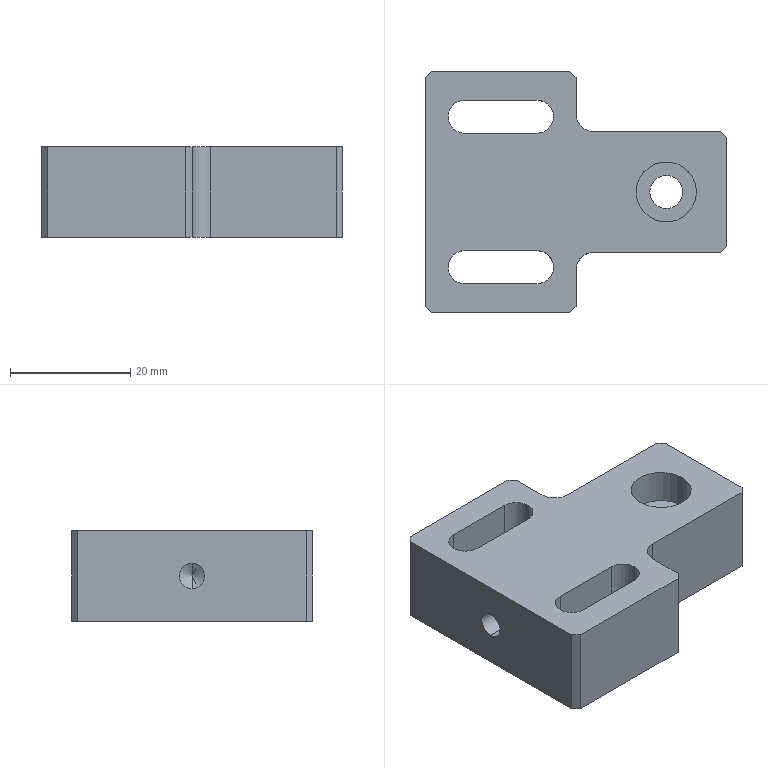Part | STEP file | MT-COMBO-119-S023 | 1 solid | 37 faces | box 50 x 40 x 15 mm | volume 18974 mm3 | plane 21 | cylinder 14 | cone 2 | commonest cylinder face diameters 5.5 x8 4.2 x2 6 x2 10 x2
STEP:
#1=CARTESIAN_POINT('',(-12.6,0.,5.4));
#2=VERTEX_POINT('',#1);
#3=CARTESIAN_POINT('',(-12.6,0.,9.6));
#4=VERTEX_POINT('',#3);
#5=CARTESIAN_POINT('',(-12.6,0.,7.5));
#6=DIRECTION('',(-1.,0.,0.));
#7=DIRECTION('',(0.,0.,1.));
#8=AXIS2_PLACEMENT_3D('',#5,#6,#7);
#9=CIRCLE('',#8,2.1);
#10=EDGE_CURVE('',#2,#4,#9,.T.);
#11=ORIENTED_EDGE('',*,*,#10,.F.);
#12=CARTESIAN_POINT('',(-25.,0.,5.4));
#13=VERTEX_POINT('',#12);
#14=CARTESIAN_POINT('',(-25.,0.,5.4));
#15=DIRECTION('',(-1.,0.,0.));
#16=VECTOR('',#15,1000.);
#17=LINE('',#14,#16);
#18=EDGE_CURVE('',#2,#13,#17,.T.);
#19=ORIENTED_EDGE('',*,*,#18,.T.);
#20=CARTESIAN_POINT('',(-25.,0.,9.6));
#21=VERTEX_POINT('',#20);
#22=CARTESIAN_POINT('',(-25.,0.,7.5));
#23=DIRECTION('',(-1.,0.,0.));
#24=DIRECTION('',(0.,0.,1.));
#25=AXIS2_PLACEMENT_3D('',#22,#23,#24);
#26=CIRCLE('',#25,2.1);
#27=EDGE_CURVE('',#13,#21,#26,.T.);
#28=ORIENTED_EDGE('',*,*,#27,.T.);
#29=CARTESIAN_POINT('',(-25.,0.,9.6));
#30=DIRECTION('',(-1.,0.,0.));
#31=VECTOR('',#30,1000.);
#32=LINE('',#29,#31);
#33=EDGE_CURVE('',#4,#21,#32,.T.);
#34=ORIENTED_EDGE('',*,*,#33,.F.);
#35=EDGE_LOOP('',(#11,#19,#28,#34));
#36=FACE_OUTER_BOUND('',#35,.T.);
#37=CARTESIAN_POINT('',(-25.,0.,7.5));
#38=DIRECTION('',(-1.,0.,0.));
#39=DIRECTION('',(0.,0.,1.));
#40=AXIS2_PLACEMENT_3D('',#37,#38,#39);
#41=CYLINDRICAL_SURFACE('',#40,2.1);
#42=ADVANCED_FACE('',(#36),#41,.F.);
#43=CARTESIAN_POINT('',(-11.338,0.,7.5));
#44=VERTEX_POINT('',#43);
#45=CARTESIAN_POINT('',(-12.6,0.,9.6));
#46=DIRECTION('',(-0.515,0.,0.8572));
#47=VECTOR('',#46,1000.);
#48=LINE('',#45,#47);
#49=EDGE_CURVE('',#44,#4,#48,.T.);
#50=ORIENTED_EDGE('',*,*,#49,.F.);
#51=CARTESIAN_POINT('',(-12.6,0.,5.4));
#52=DIRECTION('',(-0.515,0.,-0.8572));
#53=VECTOR('',#52,1000.);
#54=LINE('',#51,#53);
#55=EDGE_CURVE('',#44,#2,#54,.T.);
#56=ORIENTED_EDGE('',*,*,#55,.T.);
#57=ORIENTED_EDGE('',*,*,#10,.T.);
#58=EDGE_LOOP('',(#50,#56,#57));
#59=FACE_OUTER_BOUND('',#58,.T.);
#60=CARTESIAN_POINT('',(-12.6,0.,7.5));
#61=DIRECTION('',(-1.,0.,0.));
#62=DIRECTION('',(0.,0.,1.));
#63=AXIS2_PLACEMENT_3D('',#60,#61,#62);
#64=CONICAL_SURFACE('',#63,2.1,1.03);
#65=ADVANCED_FACE('',(#59),#64,.F.);
#66=CARTESIAN_POINT('',(-3.75,12.5,0.));
#67=VERTEX_POINT('',#66);
#68=CARTESIAN_POINT('',(-6.5,15.25,0.));
#69=VERTEX_POINT('',#68);
#70=CARTESIAN_POINT('',(-6.5,12.5,0.));
#71=DIRECTION('',(0.,0.,1.));
#72=DIRECTION('',(1.,0.,0.));
#73=AXIS2_PLACEMENT_3D('',#70,#71,#72);
#74=CIRCLE('',#73,2.75);
#75=EDGE_CURVE('',#67,#69,#74,.T.);
#76=ORIENTED_EDGE('',*,*,#75,.F.);
#77=CARTESIAN_POINT('',(-3.75,12.5,15.));
#78=VERTEX_POINT('',#77);
#79=CARTESIAN_POINT('',(-3.75,12.5,15.));
#80=DIRECTION('',(0.,0.,1.));
#81=VECTOR('',#80,1000.);
#82=LINE('',#79,#81);
#83=EDGE_CURVE('',#67,#78,#82,.T.);
#84=ORIENTED_EDGE('',*,*,#83,.T.);
#85=CARTESIAN_POINT('',(-6.5,15.25,15.));
#86=VERTEX_POINT('',#85);
#87=CARTESIAN_POINT('',(-6.5,12.5,15.));
#88=DIRECTION('',(0.,0.,1.));
#89=DIRECTION('',(1.,0.,0.));
#90=AXIS2_PLACEMENT_3D('',#87,#88,#89);
#91=CIRCLE('',#90,2.75);
#92=EDGE_CURVE('',#78,#86,#91,.T.);
#93=ORIENTED_EDGE('',*,*,#92,.T.);
#94=CARTESIAN_POINT('',(-6.5,15.25,15.));
#95=DIRECTION('',(0.,0.,1.));
#96=VECTOR('',#95,1000.);
#97=LINE('',#94,#96);
#98=EDGE_CURVE('',#69,#86,#97,.T.);
#99=ORIENTED_EDGE('',*,*,#98,.F.);
#100=EDGE_LOOP('',(#76,#84,#93,#99));
#101=FACE_OUTER_BOUND('',#100,.T.);
#102=CARTESIAN_POINT('',(-6.5,12.5,15.));
#103=DIRECTION('',(0.,0.,1.));
#104=DIRECTION('',(1.,0.,0.));
#105=AXIS2_PLACEMENT_3D('',#102,#103,#104);
#106=CYLINDRICAL_SURFACE('',#105,2.75);
#107=ADVANCED_FACE('',(#101),#106,.F.);
#108=CARTESIAN_POINT('',(-3.75,-12.5,0.));
#109=VERTEX_POINT('',#108);
#110=CARTESIAN_POINT('',(-6.5,-9.75,0.));
#111=VERTEX_POINT('',#110);
#112=CARTESIAN_POINT('',(-6.5,-12.5,0.));
#113=DIRECTION('',(0.,0.,1.));
#114=DIRECTION('',(1.,0.,0.));
#115=AXIS2_PLACEMENT_3D('',#112,#113,#114);
#116=CIRCLE('',#115,2.75);
#117=EDGE_CURVE('',#109,#111,#116,.T.);
#118=ORIENTED_EDGE('',*,*,#117,.F.);
#119=CARTESIAN_POINT('',(-3.75,-12.5,15.));
#120=VERTEX_POINT('',#119);
#121=CARTESIAN_POINT('',(-3.75,-12.5,15.));
#122=DIRECTION('',(0.,0.,1.));
#123=VECTOR('',#122,1000.);
#124=LINE('',#121,#123);
#125=EDGE_CURVE('',#109,#120,#124,.T.);
#126=ORIENTED_EDGE('',*,*,#125,.T.);
#127=CARTESIAN_POINT('',(-6.5,-9.75,15.));
#128=VERTEX_POINT('',#127);
#129=CARTESIAN_POINT('',(-6.5,-12.5,15.));
#130=DIRECTION('',(0.,0.,1.));
#131=DIRECTION('',(1.,0.,0.));
#132=AXIS2_PLACEMENT_3D('',#129,#130,#131);
#133=CIRCLE('',#132,2.75);
#134=EDGE_CURVE('',#120,#128,#133,.T.);
#135=ORIENTED_EDGE('',*,*,#134,.T.);
#136=CARTESIAN_POINT('',(-6.5,-9.75,15.));
#137=DIRECTION('',(0.,0.,1.));
#138=VECTOR('',#137,1000.);
#139=LINE('',#136,#138);
#140=EDGE_CURVE('',#111,#128,#139,.T.);
#141=ORIENTED_EDGE('',*,*,#140,.F.);
#142=EDGE_LOOP('',(#118,#126,#135,#141));
#143=FACE_OUTER_BOUND('',#142,.T.);
#144=CARTESIAN_POINT('',(-6.5,-12.5,15.));
#145=DIRECTION('',(0.,0.,1.));
#146=DIRECTION('',(1.,0.,0.));
#147=AXIS2_PLACEMENT_3D('',#144,#145,#146);
#148=CYLINDRICAL_SURFACE('',#147,2.75);
#149=ADVANCED_FACE('',(#143),#148,.F.);
#150=CARTESIAN_POINT('',(10.,0.,9.3));
#151=VERTEX_POINT('',#150);
#152=CARTESIAN_POINT('',(20.,0.,9.3));
#153=VERTEX_POINT('',#152);
#154=CARTESIAN_POINT('',(15.,0.,9.3));
#155=DIRECTION('',(0.,0.,1.));
#156=DIRECTION('',(1.,0.,0.));
#157=AXIS2_PLACEMENT_3D('',#154,#155,#156);
#158=CIRCLE('',#157,5.);
#159=EDGE_CURVE('',#151,#153,#158,.T.);
#160=ORIENTED_EDGE('',*,*,#159,.F.);
#161=CARTESIAN_POINT('',(10.,0.,15.));
#162=VERTEX_POINT('',#161);
#163=CARTESIAN_POINT('',(10.,0.,15.));
#164=DIRECTION('',(0.,0.,1.));
#165=VECTOR('',#164,1000.);
#166=LINE('',#163,#165);
#167=EDGE_CURVE('',#151,#162,#166,.T.);
#168=ORIENTED_EDGE('',*,*,#167,.T.);
#169=CARTESIAN_POINT('',(20.,0.,15.));
#170=VERTEX_POINT('',#169);
#171=CARTESIAN_POINT('',(15.,0.,15.));
#172=DIRECTION('',(0.,0.,1.));
#173=DIRECTION('',(1.,0.,0.));
#174=AXIS2_PLACEMENT_3D('',#171,#172,#173);
#175=CIRCLE('',#174,5.);
#176=EDGE_CURVE('',#162,#170,#175,.T.);
#177=ORIENTED_EDGE('',*,*,#176,.T.);
#178=CARTESIAN_POINT('',(20.,0.,15.));
#179=DIRECTION('',(0.,0.,1.));
#180=VECTOR('',#179,1000.);
#181=LINE('',#178,#180);
#182=EDGE_CURVE('',#153,#170,#181,.T.);
#183=ORIENTED_EDGE('',*,*,#182,.F.);
#184=EDGE_LOOP('',(#160,#168,#177,#183));
#185=FACE_OUTER_BOUND('',#184,.T.);
#186=CARTESIAN_POINT('',(15.,0.,15.));
#187=DIRECTION('',(0.,0.,1.));
#188=DIRECTION('',(1.,0.,0.));
#189=AXIS2_PLACEMENT_3D('',#186,#187,#188);
#190=CYLINDRICAL_SURFACE('',#189,5.);
#191=ADVANCED_FACE('',(#185),#190,.F.);
#192=CARTESIAN_POINT('',(12.25,0.,0.));
#193=VERTEX_POINT('',#192);
#194=CARTESIAN_POINT('',(17.75,0.,0.));
#195=VERTEX_POINT('',#194);
#196=CARTESIAN_POINT('',(15.,0.,0.));
#197=DIRECTION('',(0.,0.,1.));
#198=DIRECTION('',(1.,0.,0.));
#199=AXIS2_PLACEMENT_3D('',#196,#197,#198);
#200=CIRCLE('',#199,2.75);
#201=EDGE_CURVE('',#193,#195,#200,.T.);
#202=ORIENTED_EDGE('',*,*,#201,.F.);
#203=CARTESIAN_POINT('',(12.25,0.,9.3));
#204=VERTEX_POINT('',#203);
#205=CARTESIAN_POINT('',(12.25,0.,15.));
#206=DIRECTION('',(0.,0.,1.));
#207=VECTOR('',#206,1000.);
#208=LINE('',#205,#207);
#209=EDGE_CURVE('',#193,#204,#208,.T.);
#210=ORIENTED_EDGE('',*,*,#209,.T.);
#211=CARTESIAN_POINT('',(17.75,0.,9.3));
#212=VERTEX_POINT('',#211);
#213=CARTESIAN_POINT('',(15.,0.,9.3));
#214=DIRECTION('',(0.,0.,1.));
#215=DIRECTION('',(1.,0.,0.));
#216=AXIS2_PLACEMENT_3D('',#213,#214,#215);
#217=CIRCLE('',#216,2.75);
#218=EDGE_CURVE('',#204,#212,#217,.T.);
#219=ORIENTED_EDGE('',*,*,#218,.T.);
#220=CARTESIAN_POINT('',(17.75,0.,15.));
#221=DIRECTION('',(0.,0.,1.));
#222=VECTOR('',#221,1000.);
#223=LINE('',#220,#222);
#224=EDGE_CURVE('',#195,#212,#223,.T.);
#225=ORIENTED_EDGE('',*,*,#224,.F.);
#226=EDGE_LOOP('',(#202,#210,#219,#225));
#227=FACE_OUTER_BOUND('',#226,.T.);
#228=CARTESIAN_POINT('',(15.,0.,15.));
#229=DIRECTION('',(0.,0.,1.));
#230=DIRECTION('',(1.,0.,0.));
#231=AXIS2_PLACEMENT_3D('',#228,#229,#230);
#232=CYLINDRICAL_SURFACE('',#231,2.75);
#233=ADVANCED_FACE('',(#227),#232,.F.);
#234=CARTESIAN_POINT('',(25.,-9.,0.));
#235=VERTEX_POINT('',#234);
#236=CARTESIAN_POINT('',(25.,9.,0.));
#237=VERTEX_POINT('',#236);
#238=CARTESIAN_POINT('',(25.,-20.,0.));
#239=DIRECTION('',(0.,1.,0.));
#240=VECTOR('',#239,1000.);
#241=LINE('',#238,#240);
#242=EDGE_CURVE('',#235,#237,#241,.T.);
#243=ORIENTED_EDGE('',*,*,#242,.T.);
#244=CARTESIAN_POINT('',(25.,9.,15.));
#245=VERTEX_POINT('',#244);
#246=CARTESIAN_POINT('',(25.,9.,15.));
#247=DIRECTION('',(0.,0.,1.));
#248=VECTOR('',#247,1000.);
#249=LINE('',#246,#248);
#250=EDGE_CURVE('',#237,#245,#249,.T.);
#251=ORIENTED_EDGE('',*,*,#250,.T.);
#252=CARTESIAN_POINT('',(25.,-9.,15.));
#253=VERTEX_POINT('',#252);
#254=CARTESIAN_POINT('',(25.,-20.,15.));
#255=DIRECTION('',(0.,1.,0.));
#256=VECTOR('',#255,1000.);
#257=LINE('',#254,#256);
#258=EDGE_CURVE('',#253,#245,#257,.T.);
#259=ORIENTED_EDGE('',*,*,#258,.F.);
#260=CARTESIAN_POINT('',(25.,-9.,15.));
#261=DIRECTION('',(0.,0.,-1.));
#262=VECTOR('',#261,1000.);
#263=LINE('',#260,#262);
#264=EDGE_CURVE('',#253,#235,#263,.T.);
#265=ORIENTED_EDGE('',*,*,#264,.T.);
#266=EDGE_LOOP('',(#243,#251,#259,#265));
#267=FACE_OUTER_BOUND('',#266,.T.);
#268=CARTESIAN_POINT('',(25.,-20.,15.));
#269=DIRECTION('',(-1.,0.,0.));
#270=DIRECTION('',(0.,0.,1.));
#271=AXIS2_PLACEMENT_3D('',#268,#269,#270);
#272=PLANE('',#271);
#273=ADVANCED_FACE('',(#267),#272,.F.);
#274=CARTESIAN_POINT('',(-1.,20.,15.));
#275=VERTEX_POINT('',#274);
#276=CARTESIAN_POINT('',(-24.,20.,15.));
#277=VERTEX_POINT('',#276);
#278=CARTESIAN_POINT('',(-25.,20.,15.));
#279=DIRECTION('',(-1.,0.,0.));
#280=VECTOR('',#279,1000.);
#281=LINE('',#278,#280);
#282=EDGE_CURVE('',#275,#277,#281,.T.);
#283=ORIENTED_EDGE('',*,*,#282,.F.);
#284=CARTESIAN_POINT('',(-1.,20.,0.));
#285=VERTEX_POINT('',#284);
#286=CARTESIAN_POINT('',(-1.,20.,15.));
#287=DIRECTION('',(0.,0.,-1.));
#288=VECTOR('',#287,1000.);
#289=LINE('',#286,#288);
#290=EDGE_CURVE('',#275,#285,#289,.T.);
#291=ORIENTED_EDGE('',*,*,#290,.T.);
#292=CARTESIAN_POINT('',(-24.,20.,0.));
#293=VERTEX_POINT('',#292);
#294=CARTESIAN_POINT('',(-25.,20.,0.));
#295=DIRECTION('',(-1.,0.,0.));
#296=VECTOR('',#295,1000.);
#297=LINE('',#294,#296);
#298=EDGE_CURVE('',#285,#293,#297,.T.);
#299=ORIENTED_EDGE('',*,*,#298,.T.);
#300=CARTESIAN_POINT('',(-24.,20.,15.));
#301=DIRECTION('',(0.,0.,1.));
#302=VECTOR('',#301,1000.);
#303=LINE('',#300,#302);
#304=EDGE_CURVE('',#293,#277,#303,.T.);
#305=ORIENTED_EDGE('',*,*,#304,.T.);
#306=EDGE_LOOP('',(#283,#291,#299,#305));
#307=FACE_OUTER_BOUND('',#306,.T.);
#308=CARTESIAN_POINT('',(-25.,20.,15.));
#309=DIRECTION('',(0.,-1.,0.));
#310=DIRECTION('',(0.,0.,-1.));
#311=AXIS2_PLACEMENT_3D('',#308,#309,#310);
#312=PLANE('',#311);
#313=ADVANCED_FACE('',(#307),#312,.F.);
#314=CARTESIAN_POINT('',(-25.,0.,7.5));
#315=DIRECTION('',(-1.,0.,0.));
#316=DIRECTION('',(0.,0.,1.));
#317=AXIS2_PLACEMENT_3D('',#314,#315,#316);
#318=CIRCLE('',#317,2.1);
#319=EDGE_CURVE('',#21,#13,#318,.T.);
#320=ORIENTED_EDGE('',*,*,#319,.F.);
#321=ORIENTED_EDGE('',*,*,#27,.F.);
#322=EDGE_LOOP('',(#320,#321));
#323=FACE_BOUND('',#322,.T.);
#324=CARTESIAN_POINT('',(-25.,19.,15.));
#325=VERTEX_POINT('',#324);
#326=CARTESIAN_POINT('',(-25.,-19.,15.));
#327=VERTEX_POINT('',#326);
#328=CARTESIAN_POINT('',(-25.,-20.,15.));
#329=DIRECTION('',(0.,-1.,0.));
#330=VECTOR('',#329,1000.);
#331=LINE('',#328,#330);
#332=EDGE_CURVE('',#325,#327,#331,.T.);
#333=ORIENTED_EDGE('',*,*,#332,.F.);
#334=CARTESIAN_POINT('',(-25.,19.,0.));
#335=VERTEX_POINT('',#334);
#336=CARTESIAN_POINT('',(-25.,19.,15.));
#337=DIRECTION('',(0.,0.,-1.));
#338=VECTOR('',#337,1000.);
#339=LINE('',#336,#338);
#340=EDGE_CURVE('',#325,#335,#339,.T.);
#341=ORIENTED_EDGE('',*,*,#340,.T.);
#342=CARTESIAN_POINT('',(-25.,-19.,0.));
#343=VERTEX_POINT('',#342);
#344=CARTESIAN_POINT('',(-25.,-20.,0.));
#345=DIRECTION('',(0.,-1.,0.));
#346=VECTOR('',#345,1000.);
#347=LINE('',#344,#346);
#348=EDGE_CURVE('',#335,#343,#347,.T.);
#349=ORIENTED_EDGE('',*,*,#348,.T.);
#350=CARTESIAN_POINT('',(-25.,-19.,15.));
#351=DIRECTION('',(0.,0.,1.));
#352=VECTOR('',#351,1000.);
#353=LINE('',#350,#352);
#354=EDGE_CURVE('',#343,#327,#353,.T.);
#355=ORIENTED_EDGE('',*,*,#354,.T.);
#356=EDGE_LOOP('',(#333,#341,#349,#355));
#357=FACE_OUTER_BOUND('',#356,.T.);
#358=CARTESIAN_POINT('',(-25.,-20.,15.));
#359=DIRECTION('',(1.,0.,0.));
#360=DIRECTION('',(0.,0.,-1.));
#361=AXIS2_PLACEMENT_3D('',#358,#359,#360);
#362=PLANE('',#361);
#363=ADVANCED_FACE('',(#323,#357),#362,.F.);
#364=CARTESIAN_POINT('',(-24.,-20.,0.));
#365=VERTEX_POINT('',#364);
#366=CARTESIAN_POINT('',(-1.,-20.,0.));
#367=VERTEX_POINT('',#366);
#368=CARTESIAN_POINT('',(-25.,-20.,0.));
#369=DIRECTION('',(1.,0.,0.));
#370=VECTOR('',#369,1000.);
#371=LINE('',#368,#370);
#372=EDGE_CURVE('',#365,#367,#371,.T.);
#373=ORIENTED_EDGE('',*,*,#372,.T.);
#374=CARTESIAN_POINT('',(-1.,-20.,15.));
#375=VERTEX_POINT('',#374);
#376=CARTESIAN_POINT('',(-1.,-20.,15.));
#377=DIRECTION('',(0.,0.,1.));
#378=VECTOR('',#377,1000.);
#379=LINE('',#376,#378);
#380=EDGE_CURVE('',#367,#375,#379,.T.);
#381=ORIENTED_EDGE('',*,*,#380,.T.);
#382=CARTESIAN_POINT('',(-24.,-20.,15.));
#383=VERTEX_POINT('',#382);
#384=CARTESIAN_POINT('',(-25.,-20.,15.));
#385=DIRECTION('',(1.,0.,0.));
#386=VECTOR('',#385,1000.);
#387=LINE('',#384,#386);
#388=EDGE_CURVE('',#383,#375,#387,.T.);
#389=ORIENTED_EDGE('',*,*,#388,.F.);
#390=CARTESIAN_POINT('',(-24.,-20.,15.));
#391=DIRECTION('',(0.,0.,-1.));
#392=VECTOR('',#391,1000.);
#393=LINE('',#390,#392);
#394=EDGE_CURVE('',#383,#365,#393,.T.);
#395=ORIENTED_EDGE('',*,*,#394,.T.);
#396=EDGE_LOOP('',(#373,#381,#389,#395));
#397=FACE_OUTER_BOUND('',#396,.T.);
#398=CARTESIAN_POINT('',(-25.,-20.,15.));
#399=DIRECTION('',(0.,1.,0.));
#400=DIRECTION('',(0.,0.,1.));
#401=AXIS2_PLACEMENT_3D('',#398,#399,#400);
#402=PLANE('',#401);
#403=ADVANCED_FACE('',(#397),#402,.F.);
#404=CARTESIAN_POINT('',(-18.5,15.25,15.));
#405=VERTEX_POINT('',#404);
#406=CARTESIAN_POINT('',(-18.5,9.75,15.));
#407=VERTEX_POINT('',#406);
#408=CARTESIAN_POINT('',(-18.5,12.5,15.));
#409=DIRECTION('',(0.,0.,1.));
#410=DIRECTION('',(1.,0.,0.));
#411=AXIS2_PLACEMENT_3D('',#408,#409,#410);
#412=CIRCLE('',#411,2.75);
#413=EDGE_CURVE('',#405,#407,#412,.T.);
#414=ORIENTED_EDGE('',*,*,#413,.F.);
#415=CARTESIAN_POINT('',(-18.5,15.25,15.));
#416=DIRECTION('',(1.,0.,0.));
#417=VECTOR('',#416,1000.);
#418=LINE('',#415,#417);
#419=EDGE_CURVE('',#405,#86,#418,.T.);
#420=ORIENTED_EDGE('',*,*,#419,.T.);
#421=ORIENTED_EDGE('',*,*,#92,.F.);
#422=CARTESIAN_POINT('',(-6.5,9.75,15.));
#423=VERTEX_POINT('',#422);
#424=CARTESIAN_POINT('',(-6.5,12.5,15.));
#425=DIRECTION('',(0.,0.,1.));
#426=DIRECTION('',(1.,0.,0.));
#427=AXIS2_PLACEMENT_3D('',#424,#425,#426);
#428=CIRCLE('',#427,2.75);
#429=EDGE_CURVE('',#423,#78,#428,.T.);
#430=ORIENTED_EDGE('',*,*,#429,.F.);
#431=CARTESIAN_POINT('',(-18.5,9.75,15.));
#432=DIRECTION('',(1.,0.,0.));
#433=VECTOR('',#432,1000.);
#434=LINE('',#431,#433);
#435=EDGE_CURVE('',#407,#423,#434,.T.);
#436=ORIENTED_EDGE('',*,*,#435,.F.);
#437=EDGE_LOOP('',(#414,#420,#421,#430,#436));
#438=FACE_BOUND('',#437,.T.);
#439=CARTESIAN_POINT('',(-18.5,-9.75,15.));
#440=VERTEX_POINT('',#439);
#441=CARTESIAN_POINT('',(-18.5,-15.25,15.));
#442=VERTEX_POINT('',#441);
#443=CARTESIAN_POINT('',(-18.5,-12.5,15.));
#444=DIRECTION('',(0.,0.,1.));
#445=DIRECTION('',(1.,0.,0.));
#446=AXIS2_PLACEMENT_3D('',#443,#444,#445);
#447=CIRCLE('',#446,2.75);
#448=EDGE_CURVE('',#440,#442,#447,.T.);
#449=ORIENTED_EDGE('',*,*,#448,.F.);
#450=CARTESIAN_POINT('',(-18.5,-9.75,15.));
#451=DIRECTION('',(1.,0.,0.));
#452=VECTOR('',#451,1000.);
#453=LINE('',#450,#452);
#454=EDGE_CURVE('',#440,#128,#453,.T.);
#455=ORIENTED_EDGE('',*,*,#454,.T.);
#456=ORIENTED_EDGE('',*,*,#134,.F.);
#457=CARTESIAN_POINT('',(-6.5,-15.25,15.));
#458=VERTEX_POINT('',#457);
#459=CARTESIAN_POINT('',(-6.5,-12.5,15.));
#460=DIRECTION('',(0.,0.,1.));
#461=DIRECTION('',(1.,0.,0.));
#462=AXIS2_PLACEMENT_3D('',#459,#460,#461);
#463=CIRCLE('',#462,2.75);
#464=EDGE_CURVE('',#458,#120,#463,.T.);
#465=ORIENTED_EDGE('',*,*,#464,.F.);
#466=CARTESIAN_POINT('',(-18.5,-15.25,15.));
#467=DIRECTION('',(1.,0.,0.));
#468=VECTOR('',#467,1000.);
#469=LINE('',#466,#468);
#470=EDGE_CURVE('',#442,#458,#469,.T.);
#471=ORIENTED_EDGE('',*,*,#470,.F.);
#472=EDGE_LOOP('',(#449,#455,#456,#465,#471));
#473=FACE_BOUND('',#472,.T.);
#474=CARTESIAN_POINT('',(15.,0.,15.));
#475=DIRECTION('',(0.,0.,1.));
#476=DIRECTION('',(1.,0.,0.));
#477=AXIS2_PLACEMENT_3D('',#474,#475,#476);
#478=CIRCLE('',#477,5.);
#479=EDGE_CURVE('',#170,#162,#478,.T.);
#480=ORIENTED_EDGE('',*,*,#479,.F.);
#481=ORIENTED_EDGE('',*,*,#176,.F.);
#482=EDGE_LOOP('',(#480,#481));
#483=FACE_BOUND('',#482,.T.);
#484=CARTESIAN_POINT('',(0.,19.,15.));
#485=VERTEX_POINT('',#484);
#486=CARTESIAN_POINT('',(0.,13.,15.));
#487=VERTEX_POINT('',#486);
#488=CARTESIAN_POINT('',(0.,20.,15.));
#489=DIRECTION('',(0.,-1.,0.));
#490=VECTOR('',#489,1000.);
#491=LINE('',#488,#490);
#492=EDGE_CURVE('',#485,#487,#491,.T.);
#493=ORIENTED_EDGE('',*,*,#492,.F.);
#494=CARTESIAN_POINT('',(0.,19.,15.));
#495=DIRECTION('',(-0.7071,0.7071,0.));
#496=VECTOR('',#495,1000.);
#497=LINE('',#494,#496);
#498=EDGE_CURVE('',#485,#275,#497,.T.);
#499=ORIENTED_EDGE('',*,*,#498,.T.);
#500=ORIENTED_EDGE('',*,*,#282,.T.);
#501=CARTESIAN_POINT('',(-25.,19.,15.));
#502=DIRECTION('',(-0.7071,-0.7071,0.));
#503=VECTOR('',#502,1000.);
#504=LINE('',#501,#503);
#505=EDGE_CURVE('',#277,#325,#504,.T.);
#506=ORIENTED_EDGE('',*,*,#505,.T.);
#507=ORIENTED_EDGE('',*,*,#332,.T.);
#508=CARTESIAN_POINT('',(-24.,-20.,15.));
#509=DIRECTION('',(0.7071,-0.7071,0.));
#510=VECTOR('',#509,1000.);
#511=LINE('',#508,#510);
#512=EDGE_CURVE('',#327,#383,#511,.T.);
#513=ORIENTED_EDGE('',*,*,#512,.T.);
#514=ORIENTED_EDGE('',*,*,#388,.T.);
#515=CARTESIAN_POINT('',(0.,-19.,15.));
#516=VERTEX_POINT('',#515);
#517=CARTESIAN_POINT('',(-1.,-20.,15.));
#518=DIRECTION('',(0.7071,0.7071,0.));
#519=VECTOR('',#518,1000.);
#520=LINE('',#517,#519);
#521=EDGE_CURVE('',#375,#516,#520,.T.);
#522=ORIENTED_EDGE('',*,*,#521,.T.);
#523=CARTESIAN_POINT('',(0.,-13.,15.));
#524=VERTEX_POINT('',#523);
#525=CARTESIAN_POINT('',(0.,-20.,15.));
#526=DIRECTION('',(0.,-1.,0.));
#527=VECTOR('',#526,1000.);
#528=LINE('',#525,#527);
#529=EDGE_CURVE('',#524,#516,#528,.T.);
#530=ORIENTED_EDGE('',*,*,#529,.F.);
#531=CARTESIAN_POINT('',(3.,-10.,15.));
#532=VERTEX_POINT('',#531);
#533=CARTESIAN_POINT('',(3.,-13.,15.));
#534=DIRECTION('',(0.,0.,-1.));
#535=DIRECTION('',(-1.,0.,0.));
#536=AXIS2_PLACEMENT_3D('',#533,#534,#535);
#537=CIRCLE('',#536,3.);
#538=EDGE_CURVE('',#524,#532,#537,.T.);
#539=ORIENTED_EDGE('',*,*,#538,.T.);
#540=CARTESIAN_POINT('',(24.,-10.,15.));
#541=VERTEX_POINT('',#540);
#542=CARTESIAN_POINT('',(25.,-10.,15.));
#543=DIRECTION('',(-1.,0.,0.));
#544=VECTOR('',#543,1000.);
#545=LINE('',#542,#544);
#546=EDGE_CURVE('',#541,#532,#545,.T.);
#547=ORIENTED_EDGE('',*,*,#546,.F.);
#548=CARTESIAN_POINT('',(24.,-10.,15.));
#549=DIRECTION('',(0.7071,0.7071,0.));
#550=VECTOR('',#549,1000.);
#551=LINE('',#548,#550);
#552=EDGE_CURVE('',#541,#253,#551,.T.);
#553=ORIENTED_EDGE('',*,*,#552,.T.);
#554=ORIENTED_EDGE('',*,*,#258,.T.);
#555=CARTESIAN_POINT('',(24.,10.,15.));
#556=VERTEX_POINT('',#555);
#557=CARTESIAN_POINT('',(25.,9.,15.));
#558=DIRECTION('',(-0.7071,0.7071,0.));
#559=VECTOR('',#558,1000.);
#560=LINE('',#557,#559);
#561=EDGE_CURVE('',#245,#556,#560,.T.);
#562=ORIENTED_EDGE('',*,*,#561,.T.);
#563=CARTESIAN_POINT('',(3.,10.,15.));
#564=VERTEX_POINT('',#563);
#565=CARTESIAN_POINT('',(25.,10.,15.));
#566=DIRECTION('',(1.,0.,0.));
#567=VECTOR('',#566,1000.);
#568=LINE('',#565,#567);
#569=EDGE_CURVE('',#564,#556,#568,.T.);
#570=ORIENTED_EDGE('',*,*,#569,.F.);
#571=CARTESIAN_POINT('',(3.,13.,15.));
#572=DIRECTION('',(0.,0.,-1.));
#573=DIRECTION('',(-1.,0.,0.));
#574=AXIS2_PLACEMENT_3D('',#571,#572,#573);
#575=CIRCLE('',#574,3.);
#576=EDGE_CURVE('',#564,#487,#575,.T.);
#577=ORIENTED_EDGE('',*,*,#576,.T.);
#578=EDGE_LOOP('',(#493,#499,#500,#506,#507,#513,#514,#522,#530,#539,#547,#553,#554,#562,#570,#577));
#579=FACE_OUTER_BOUND('',#578,.T.);
#580=CARTESIAN_POINT('',(0.,0.,15.));
#581=DIRECTION('',(0.,0.,-1.));
#582=DIRECTION('',(-1.,0.,0.));
#583=AXIS2_PLACEMENT_3D('',#580,#581,#582);
#584=PLANE('',#583);
#585=ADVANCED_FACE('',(#438,#473,#483,#579),#584,.F.);
#586=CARTESIAN_POINT('',(-18.5,15.25,0.));
#587=VERTEX_POINT('',#586);
#588=CARTESIAN_POINT('',(-18.5,15.25,0.));
#589=DIRECTION('',(1.,0.,0.));
#590=VECTOR('',#589,1000.);
#591=LINE('',#588,#590);
#592=EDGE_CURVE('',#587,#69,#591,.T.);
#593=ORIENTED_EDGE('',*,*,#592,.F.);
#594=CARTESIAN_POINT('',(-18.5,9.75,0.));
#595=VERTEX_POINT('',#594);
#596=CARTESIAN_POINT('',(-18.5,12.5,0.));
#597=DIRECTION('',(0.,0.,1.));
#598=DIRECTION('',(1.,0.,0.));
#599=AXIS2_PLACEMENT_3D('',#596,#597,#598);
#600=CIRCLE('',#599,2.75);
#601=EDGE_CURVE('',#587,#595,#600,.T.);
#602=ORIENTED_EDGE('',*,*,#601,.T.);
#603=CARTESIAN_POINT('',(-6.5,9.75,0.));
#604=VERTEX_POINT('',#603);
#605=CARTESIAN_POINT('',(-18.5,9.75,0.));
#606=DIRECTION('',(1.,0.,0.));
#607=VECTOR('',#606,1000.);
#608=LINE('',#605,#607);
#609=EDGE_CURVE('',#595,#604,#608,.T.);
#610=ORIENTED_EDGE('',*,*,#609,.T.);
#611=CARTESIAN_POINT('',(-6.5,12.5,0.));
#612=DIRECTION('',(0.,0.,1.));
#613=DIRECTION('',(1.,0.,0.));
#614=AXIS2_PLACEMENT_3D('',#611,#612,#613);
#615=CIRCLE('',#614,2.75);
#616=EDGE_CURVE('',#604,#67,#615,.T.);
#617=ORIENTED_EDGE('',*,*,#616,.T.);
#618=ORIENTED_EDGE('',*,*,#75,.T.);
#619=EDGE_LOOP('',(#593,#602,#610,#617,#618));
#620=FACE_BOUND('',#619,.T.);
#621=CARTESIAN_POINT('',(-6.5,-15.25,0.));
#622=VERTEX_POINT('',#621);
#623=CARTESIAN_POINT('',(-6.5,-12.5,0.));
#624=DIRECTION('',(0.,0.,1.));
#625=DIRECTION('',(1.,0.,0.));
#626=AXIS2_PLACEMENT_3D('',#623,#624,#625);
#627=CIRCLE('',#626,2.75);
#628=EDGE_CURVE('',#622,#109,#627,.T.);
#629=ORIENTED_EDGE('',*,*,#628,.T.);
#630=ORIENTED_EDGE('',*,*,#117,.T.);
#631=CARTESIAN_POINT('',(-18.5,-9.75,0.));
#632=VERTEX_POINT('',#631);
#633=CARTESIAN_POINT('',(-18.5,-9.75,0.));
#634=DIRECTION('',(1.,0.,0.));
#635=VECTOR('',#634,1000.);
#636=LINE('',#633,#635);
#637=EDGE_CURVE('',#632,#111,#636,.T.);
#638=ORIENTED_EDGE('',*,*,#637,.F.);
#639=CARTESIAN_POINT('',(-18.5,-15.25,0.));
#640=VERTEX_POINT('',#639);
#641=CARTESIAN_POINT('',(-18.5,-12.5,0.));
#642=DIRECTION('',(0.,0.,1.));
#643=DIRECTION('',(1.,0.,0.));
#644=AXIS2_PLACEMENT_3D('',#641,#642,#643);
#645=CIRCLE('',#644,2.75);
#646=EDGE_CURVE('',#632,#640,#645,.T.);
#647=ORIENTED_EDGE('',*,*,#646,.T.);
#648=CARTESIAN_POINT('',(-18.5,-15.25,0.));
#649=DIRECTION('',(1.,0.,0.));
#650=VECTOR('',#649,1000.);
#651=LINE('',#648,#650);
#652=EDGE_CURVE('',#640,#622,#651,.T.);
#653=ORIENTED_EDGE('',*,*,#652,.T.);
#654=EDGE_LOOP('',(#629,#630,#638,#647,#653));
#655=FACE_BOUND('',#654,.T.);
#656=ORIENTED_EDGE('',*,*,#298,.F.);
#657=CARTESIAN_POINT('',(0.,19.,0.));
#658=VERTEX_POINT('',#657);
#659=CARTESIAN_POINT('',(9.5,9.5,0.));
#660=DIRECTION('',(0.7071,-0.7071,0.));
#661=VECTOR('',#660,1000.);
#662=LINE('',#659,#661);
#663=EDGE_CURVE('',#285,#658,#662,.T.);
#664=ORIENTED_EDGE('',*,*,#663,.T.);
#665=CARTESIAN_POINT('',(0.,13.,0.));
#666=VERTEX_POINT('',#665);
#667=CARTESIAN_POINT('',(0.,20.,0.));
#668=DIRECTION('',(0.,-1.,0.));
#669=VECTOR('',#668,1000.);
#670=LINE('',#667,#669);
#671=EDGE_CURVE('',#658,#666,#670,.T.);
#672=ORIENTED_EDGE('',*,*,#671,.T.);
#673=CARTESIAN_POINT('',(3.,10.,0.));
#674=VERTEX_POINT('',#673);
#675=CARTESIAN_POINT('',(3.,13.,0.));
#676=DIRECTION('',(0.,0.,1.));
#677=DIRECTION('',(-1.,0.,0.));
#678=AXIS2_PLACEMENT_3D('',#675,#676,#677);
#679=CIRCLE('',#678,3.);
#680=EDGE_CURVE('',#666,#674,#679,.T.);
#681=ORIENTED_EDGE('',*,*,#680,.T.);
#682=CARTESIAN_POINT('',(24.,10.,0.));
#683=VERTEX_POINT('',#682);
#684=CARTESIAN_POINT('',(25.,10.,0.));
#685=DIRECTION('',(1.,0.,0.));
#686=VECTOR('',#685,1000.);
#687=LINE('',#684,#686);
#688=EDGE_CURVE('',#674,#683,#687,.T.);
#689=ORIENTED_EDGE('',*,*,#688,.T.);
#690=CARTESIAN_POINT('',(17.,17.,0.));
#691=DIRECTION('',(0.7071,-0.7071,0.));
#692=VECTOR('',#691,1000.);
#693=LINE('',#690,#692);
#694=EDGE_CURVE('',#683,#237,#693,.T.);
#695=ORIENTED_EDGE('',*,*,#694,.T.);
#696=ORIENTED_EDGE('',*,*,#242,.F.);
#697=CARTESIAN_POINT('',(24.,-10.,0.));
#698=VERTEX_POINT('',#697);
#699=CARTESIAN_POINT('',(17.,-17.,0.));
#700=DIRECTION('',(-0.7071,-0.7071,0.));
#701=VECTOR('',#700,1000.);
#702=LINE('',#699,#701);
#703=EDGE_CURVE('',#235,#698,#702,.T.);
#704=ORIENTED_EDGE('',*,*,#703,.T.);
#705=CARTESIAN_POINT('',(3.,-10.,0.));
#706=VERTEX_POINT('',#705);
#707=CARTESIAN_POINT('',(25.,-10.,0.));
#708=DIRECTION('',(-1.,0.,0.));
#709=VECTOR('',#708,1000.);
#710=LINE('',#707,#709);
#711=EDGE_CURVE('',#698,#706,#710,.T.);
#712=ORIENTED_EDGE('',*,*,#711,.T.);
#713=CARTESIAN_POINT('',(0.,-13.,0.));
#714=VERTEX_POINT('',#713);
#715=CARTESIAN_POINT('',(3.,-13.,0.));
#716=DIRECTION('',(0.,0.,1.));
#717=DIRECTION('',(-1.,0.,0.));
#718=AXIS2_PLACEMENT_3D('',#715,#716,#717);
#719=CIRCLE('',#718,3.);
#720=EDGE_CURVE('',#706,#714,#719,.T.);
#721=ORIENTED_EDGE('',*,*,#720,.T.);
#722=CARTESIAN_POINT('',(0.,-19.,0.));
#723=VERTEX_POINT('',#722);
#724=CARTESIAN_POINT('',(0.,-20.,0.));
#725=DIRECTION('',(0.,-1.,0.));
#726=VECTOR('',#725,1000.);
#727=LINE('',#724,#726);
#728=EDGE_CURVE('',#714,#723,#727,.T.);
#729=ORIENTED_EDGE('',*,*,#728,.T.);
#730=CARTESIAN_POINT('',(9.5,-9.5,0.));
#731=DIRECTION('',(-0.7071,-0.7071,0.));
#732=VECTOR('',#731,1000.);
#733=LINE('',#730,#732);
#734=EDGE_CURVE('',#723,#367,#733,.T.);
#735=ORIENTED_EDGE('',*,*,#734,.T.);
#736=ORIENTED_EDGE('',*,*,#372,.F.);
#737=CARTESIAN_POINT('',(-22.,-22.,0.));
#738=DIRECTION('',(-0.7071,0.7071,0.));
#739=VECTOR('',#738,1000.);
#740=LINE('',#737,#739);
#741=EDGE_CURVE('',#365,#343,#740,.T.);
#742=ORIENTED_EDGE('',*,*,#741,.T.);
#743=ORIENTED_EDGE('',*,*,#348,.F.);
#744=CARTESIAN_POINT('',(-22.,22.,0.));
#745=DIRECTION('',(0.7071,0.7071,0.));
#746=VECTOR('',#745,1000.);
#747=LINE('',#744,#746);
#748=EDGE_CURVE('',#335,#293,#747,.T.);
#749=ORIENTED_EDGE('',*,*,#748,.T.);
#750=EDGE_LOOP('',(#656,#664,#672,#681,#689,#695,#696,#704,#712,#721,#729,#735,#736,#742,#743,#749));
#751=FACE_OUTER_BOUND('',#750,.T.);
#752=CARTESIAN_POINT('',(15.,0.,0.));
#753=DIRECTION('',(0.,0.,1.));
#754=DIRECTION('',(1.,0.,0.));
#755=AXIS2_PLACEMENT_3D('',#752,#753,#754);
#756=CIRCLE('',#755,2.75);
#757=EDGE_CURVE('',#195,#193,#756,.T.);
#758=ORIENTED_EDGE('',*,*,#757,.T.);
#759=ORIENTED_EDGE('',*,*,#201,.T.);
#760=EDGE_LOOP('',(#758,#759));
#761=FACE_BOUND('',#760,.T.);
#762=CARTESIAN_POINT('',(0.,0.,0.));
#763=DIRECTION('',(0.,0.,-1.));
#764=DIRECTION('',(-1.,0.,0.));
#765=AXIS2_PLACEMENT_3D('',#762,#763,#764);
#766=PLANE('',#765);
#767=ADVANCED_FACE('',(#620,#655,#751,#761),#766,.T.);
#768=ORIENTED_EDGE('',*,*,#209,.F.);
#769=ORIENTED_EDGE('',*,*,#757,.F.);
#770=ORIENTED_EDGE('',*,*,#224,.T.);
#771=CARTESIAN_POINT('',(15.,0.,9.3));
#772=DIRECTION('',(0.,0.,1.));
#773=DIRECTION('',(1.,0.,0.));
#774=AXIS2_PLACEMENT_3D('',#771,#772,#773);
#775=CIRCLE('',#774,2.75);
#776=EDGE_CURVE('',#212,#204,#775,.T.);
#777=ORIENTED_EDGE('',*,*,#776,.T.);
#778=EDGE_LOOP('',(#768,#769,#770,#777));
#779=FACE_OUTER_BOUND('',#778,.T.);
#780=CARTESIAN_POINT('',(15.,0.,15.));
#781=DIRECTION('',(0.,0.,1.));
#782=DIRECTION('',(1.,0.,0.));
#783=AXIS2_PLACEMENT_3D('',#780,#781,#782);
#784=CYLINDRICAL_SURFACE('',#783,2.75);
#785=ADVANCED_FACE('',(#779),#784,.F.);
#786=ORIENTED_EDGE('',*,*,#776,.F.);
#787=ORIENTED_EDGE('',*,*,#218,.F.);
#788=EDGE_LOOP('',(#786,#787));
#789=FACE_BOUND('',#788,.T.);
#790=CARTESIAN_POINT('',(15.,0.,9.3));
#791=DIRECTION('',(0.,0.,1.));
#792=DIRECTION('',(1.,0.,0.));
#793=AXIS2_PLACEMENT_3D('',#790,#791,#792);
#794=CIRCLE('',#793,5.);
#795=EDGE_CURVE('',#153,#151,#794,.T.);
#796=ORIENTED_EDGE('',*,*,#795,.T.);
#797=ORIENTED_EDGE('',*,*,#159,.T.);
#798=EDGE_LOOP('',(#796,#797));
#799=FACE_OUTER_BOUND('',#798,.T.);
#800=CARTESIAN_POINT('',(17.75,0.,9.3));
#801=DIRECTION('',(0.,0.,-1.));
#802=DIRECTION('',(-1.,0.,0.));
#803=AXIS2_PLACEMENT_3D('',#800,#801,#802);
#804=PLANE('',#803);
#805=ADVANCED_FACE('',(#789,#799),#804,.F.);
#806=ORIENTED_EDGE('',*,*,#167,.F.);
#807=ORIENTED_EDGE('',*,*,#795,.F.);
#808=ORIENTED_EDGE('',*,*,#182,.T.);
#809=ORIENTED_EDGE('',*,*,#479,.T.);
#810=EDGE_LOOP('',(#806,#807,#808,#809));
#811=FACE_OUTER_BOUND('',#810,.T.);
#812=CARTESIAN_POINT('',(15.,0.,15.));
#813=DIRECTION('',(0.,0.,1.));
#814=DIRECTION('',(1.,0.,0.));
#815=AXIS2_PLACEMENT_3D('',#812,#813,#814);
#816=CYLINDRICAL_SURFACE('',#815,5.);
#817=ADVANCED_FACE('',(#811),#816,.F.);
#818=ORIENTED_EDGE('',*,*,#728,.F.);
#819=CARTESIAN_POINT('',(0.,-13.,15.));
#820=DIRECTION('',(0.,0.,1.));
#821=VECTOR('',#820,1000.);
#822=LINE('',#819,#821);
#823=EDGE_CURVE('',#714,#524,#822,.T.);
#824=ORIENTED_EDGE('',*,*,#823,.T.);
#825=ORIENTED_EDGE('',*,*,#529,.T.);
#826=CARTESIAN_POINT('',(0.,-19.,0.));
#827=DIRECTION('',(0.,0.,-1.));
#828=VECTOR('',#827,1000.);
#829=LINE('',#826,#828);
#830=EDGE_CURVE('',#516,#723,#829,.T.);
#831=ORIENTED_EDGE('',*,*,#830,.T.);
#832=EDGE_LOOP('',(#818,#824,#825,#831));
#833=FACE_OUTER_BOUND('',#832,.T.);
#834=CARTESIAN_POINT('',(0.,-20.,0.));
#835=DIRECTION('',(-1.,0.,0.));
#836=DIRECTION('',(0.,0.,1.));
#837=AXIS2_PLACEMENT_3D('',#834,#835,#836);
#838=PLANE('',#837);
#839=ADVANCED_FACE('',(#833),#838,.F.);
#840=ORIENTED_EDGE('',*,*,#546,.T.);
#841=CARTESIAN_POINT('',(3.,-10.,0.));
#842=DIRECTION('',(0.,0.,-1.));
#843=VECTOR('',#842,1000.);
#844=LINE('',#841,#843);
#845=EDGE_CURVE('',#532,#706,#844,.T.);
#846=ORIENTED_EDGE('',*,*,#845,.T.);
#847=ORIENTED_EDGE('',*,*,#711,.F.);
#848=CARTESIAN_POINT('',(24.,-10.,0.));
#849=DIRECTION('',(0.,0.,1.));
#850=VECTOR('',#849,1000.);
#851=LINE('',#848,#850);
#852=EDGE_CURVE('',#698,#541,#851,.T.);
#853=ORIENTED_EDGE('',*,*,#852,.T.);
#854=EDGE_LOOP('',(#840,#846,#847,#853));
#855=FACE_OUTER_BOUND('',#854,.T.);
#856=CARTESIAN_POINT('',(25.,-10.,0.));
#857=DIRECTION('',(0.,1.,0.));
#858=DIRECTION('',(-1.,0.,0.));
#859=AXIS2_PLACEMENT_3D('',#856,#857,#858);
#860=PLANE('',#859);
#861=ADVANCED_FACE('',(#855),#860,.F.);
#862=ORIENTED_EDGE('',*,*,#688,.F.);
#863=CARTESIAN_POINT('',(3.,10.,15.));
#864=DIRECTION('',(0.,0.,1.));
#865=VECTOR('',#864,1000.);
#866=LINE('',#863,#865);
#867=EDGE_CURVE('',#674,#564,#866,.T.);
#868=ORIENTED_EDGE('',*,*,#867,.T.);
#869=ORIENTED_EDGE('',*,*,#569,.T.);
#870=CARTESIAN_POINT('',(24.,10.,0.));
#871=DIRECTION('',(0.,0.,-1.));
#872=VECTOR('',#871,1000.);
#873=LINE('',#870,#872);
#874=EDGE_CURVE('',#556,#683,#873,.T.);
#875=ORIENTED_EDGE('',*,*,#874,.T.);
#876=EDGE_LOOP('',(#862,#868,#869,#875));
#877=FACE_OUTER_BOUND('',#876,.T.);
#878=CARTESIAN_POINT('',(25.,10.,0.));
#879=DIRECTION('',(0.,-1.,0.));
#880=DIRECTION('',(1.,0.,0.));
#881=AXIS2_PLACEMENT_3D('',#878,#879,#880);
#882=PLANE('',#881);
#883=ADVANCED_FACE('',(#877),#882,.F.);
#884=ORIENTED_EDGE('',*,*,#492,.T.);
#885=CARTESIAN_POINT('',(0.,13.,0.));
#886=DIRECTION('',(0.,0.,-1.));
#887=VECTOR('',#886,1000.);
#888=LINE('',#885,#887);
#889=EDGE_CURVE('',#487,#666,#888,.T.);
#890=ORIENTED_EDGE('',*,*,#889,.T.);
#891=ORIENTED_EDGE('',*,*,#671,.F.);
#892=CARTESIAN_POINT('',(0.,19.,0.));
#893=DIRECTION('',(0.,0.,1.));
#894=VECTOR('',#893,1000.);
#895=LINE('',#892,#894);
#896=EDGE_CURVE('',#658,#485,#895,.T.);
#897=ORIENTED_EDGE('',*,*,#896,.T.);
#898=EDGE_LOOP('',(#884,#890,#891,#897));
#899=FACE_OUTER_BOUND('',#898,.T.);
#900=CARTESIAN_POINT('',(0.,20.,0.));
#901=DIRECTION('',(-1.,0.,0.));
#902=DIRECTION('',(0.,0.,1.));
#903=AXIS2_PLACEMENT_3D('',#900,#901,#902);
#904=PLANE('',#903);
#905=ADVANCED_FACE('',(#899),#904,.F.);
#906=ORIENTED_EDGE('',*,*,#125,.F.);
#907=ORIENTED_EDGE('',*,*,#628,.F.);
#908=CARTESIAN_POINT('',(-6.5,-15.25,15.));
#909=DIRECTION('',(0.,0.,-1.));
#910=VECTOR('',#909,1000.);
#911=LINE('',#908,#910);
#912=EDGE_CURVE('',#458,#622,#911,.T.);
#913=ORIENTED_EDGE('',*,*,#912,.F.);
#914=ORIENTED_EDGE('',*,*,#464,.T.);
#915=EDGE_LOOP('',(#906,#907,#913,#914));
#916=FACE_OUTER_BOUND('',#915,.T.);
#917=CARTESIAN_POINT('',(-6.5,-12.5,15.));
#918=DIRECTION('',(0.,0.,1.));
#919=DIRECTION('',(1.,0.,0.));
#920=AXIS2_PLACEMENT_3D('',#917,#918,#919);
#921=CYLINDRICAL_SURFACE('',#920,2.75);
#922=ADVANCED_FACE('',(#916),#921,.F.);
#923=ORIENTED_EDGE('',*,*,#448,.T.);
#924=CARTESIAN_POINT('',(-18.5,-15.25,15.));
#925=DIRECTION('',(0.,0.,1.));
#926=VECTOR('',#925,1000.);
#927=LINE('',#924,#926);
#928=EDGE_CURVE('',#640,#442,#927,.T.);
#929=ORIENTED_EDGE('',*,*,#928,.F.);
#930=ORIENTED_EDGE('',*,*,#646,.F.);
#931=CARTESIAN_POINT('',(-18.5,-9.75,15.));
#932=DIRECTION('',(0.,0.,-1.));
#933=VECTOR('',#932,1000.);
#934=LINE('',#931,#933);
#935=EDGE_CURVE('',#440,#632,#934,.T.);
#936=ORIENTED_EDGE('',*,*,#935,.F.);
#937=EDGE_LOOP('',(#923,#929,#930,#936));
#938=FACE_OUTER_BOUND('',#937,.T.);
#939=CARTESIAN_POINT('',(-18.5,-12.5,15.));
#940=DIRECTION('',(0.,0.,1.));
#941=DIRECTION('',(1.,0.,0.));
#942=AXIS2_PLACEMENT_3D('',#939,#940,#941);
#943=CYLINDRICAL_SURFACE('',#942,2.75);
#944=ADVANCED_FACE('',(#938),#943,.F.);
#945=ORIENTED_EDGE('',*,*,#140,.T.);
#946=ORIENTED_EDGE('',*,*,#454,.F.);
#947=ORIENTED_EDGE('',*,*,#935,.T.);
#948=ORIENTED_EDGE('',*,*,#637,.T.);
#949=EDGE_LOOP('',(#945,#946,#947,#948));
#950=FACE_OUTER_BOUND('',#949,.T.);
#951=CARTESIAN_POINT('',(-18.5,-9.75,15.));
#952=DIRECTION('',(0.,1.,0.));
#953=DIRECTION('',(0.,0.,1.));
#954=AXIS2_PLACEMENT_3D('',#951,#952,#953);
#955=PLANE('',#954);
#956=ADVANCED_FACE('',(#950),#955,.F.);
#957=ORIENTED_EDGE('',*,*,#912,.T.);
#958=ORIENTED_EDGE('',*,*,#652,.F.);
#959=ORIENTED_EDGE('',*,*,#928,.T.);
#960=ORIENTED_EDGE('',*,*,#470,.T.);
#961=EDGE_LOOP('',(#957,#958,#959,#960));
#962=FACE_OUTER_BOUND('',#961,.T.);
#963=CARTESIAN_POINT('',(-18.5,-15.25,15.));
#964=DIRECTION('',(0.,-1.,0.));
#965=DIRECTION('',(0.,0.,-1.));
#966=AXIS2_PLACEMENT_3D('',#963,#964,#965);
#967=PLANE('',#966);
#968=ADVANCED_FACE('',(#962),#967,.F.);
#969=ORIENTED_EDGE('',*,*,#83,.F.);
#970=ORIENTED_EDGE('',*,*,#616,.F.);
#971=CARTESIAN_POINT('',(-6.5,9.75,15.));
#972=DIRECTION('',(0.,0.,-1.));
#973=VECTOR('',#972,1000.);
#974=LINE('',#971,#973);
#975=EDGE_CURVE('',#423,#604,#974,.T.);
#976=ORIENTED_EDGE('',*,*,#975,.F.);
#977=ORIENTED_EDGE('',*,*,#429,.T.);
#978=EDGE_LOOP('',(#969,#970,#976,#977));
#979=FACE_OUTER_BOUND('',#978,.T.);
#980=CARTESIAN_POINT('',(-6.5,12.5,15.));
#981=DIRECTION('',(0.,0.,1.));
#982=DIRECTION('',(1.,0.,0.));
#983=AXIS2_PLACEMENT_3D('',#980,#981,#982);
#984=CYLINDRICAL_SURFACE('',#983,2.75);
#985=ADVANCED_FACE('',(#979),#984,.F.);
#986=ORIENTED_EDGE('',*,*,#413,.T.);
#987=CARTESIAN_POINT('',(-18.5,9.75,15.));
#988=DIRECTION('',(0.,0.,1.));
#989=VECTOR('',#988,1000.);
#990=LINE('',#987,#989);
#991=EDGE_CURVE('',#595,#407,#990,.T.);
#992=ORIENTED_EDGE('',*,*,#991,.F.);
#993=ORIENTED_EDGE('',*,*,#601,.F.);
#994=CARTESIAN_POINT('',(-18.5,15.25,15.));
#995=DIRECTION('',(0.,0.,-1.));
#996=VECTOR('',#995,1000.);
#997=LINE('',#994,#996);
#998=EDGE_CURVE('',#405,#587,#997,.T.);
#999=ORIENTED_EDGE('',*,*,#998,.F.);
#1000=EDGE_LOOP('',(#986,#992,#993,#999));
#1001=FACE_OUTER_BOUND('',#1000,.T.);
#1002=CARTESIAN_POINT('',(-18.5,12.5,15.));
#1003=DIRECTION('',(0.,0.,1.));
#1004=DIRECTION('',(1.,0.,0.));
#1005=AXIS2_PLACEMENT_3D('',#1002,#1003,#1004);
#1006=CYLINDRICAL_SURFACE('',#1005,2.75);
#1007=ADVANCED_FACE('',(#1001),#1006,.F.);
#1008=ORIENTED_EDGE('',*,*,#98,.T.);
#1009=ORIENTED_EDGE('',*,*,#419,.F.);
#1010=ORIENTED_EDGE('',*,*,#998,.T.);
#1011=ORIENTED_EDGE('',*,*,#592,.T.);
#1012=EDGE_LOOP('',(#1008,#1009,#1010,#1011));
#1013=FACE_OUTER_BOUND('',#1012,.T.);
#1014=CARTESIAN_POINT('',(-18.5,15.25,15.));
#1015=DIRECTION('',(0.,1.,0.));
#1016=DIRECTION('',(0.,0.,1.));
#1017=AXIS2_PLACEMENT_3D('',#1014,#1015,#1016);
#1018=PLANE('',#1017);
#1019=ADVANCED_FACE('',(#1013),#1018,.F.);
#1020=ORIENTED_EDGE('',*,*,#975,.T.);
#1021=ORIENTED_EDGE('',*,*,#609,.F.);
#1022=ORIENTED_EDGE('',*,*,#991,.T.);
#1023=ORIENTED_EDGE('',*,*,#435,.T.);
#1024=EDGE_LOOP('',(#1020,#1021,#1022,#1023));
#1025=FACE_OUTER_BOUND('',#1024,.T.);
#1026=CARTESIAN_POINT('',(-18.5,9.75,15.));
#1027=DIRECTION('',(0.,-1.,0.));
#1028=DIRECTION('',(0.,0.,-1.));
#1029=AXIS2_PLACEMENT_3D('',#1026,#1027,#1028);
#1030=PLANE('',#1029);
#1031=ADVANCED_FACE('',(#1025),#1030,.F.);
#1032=ORIENTED_EDGE('',*,*,#663,.F.);
#1033=ORIENTED_EDGE('',*,*,#290,.F.);
#1034=ORIENTED_EDGE('',*,*,#498,.F.);
#1035=ORIENTED_EDGE('',*,*,#896,.F.);
#1036=EDGE_LOOP('',(#1032,#1033,#1034,#1035));
#1037=FACE_OUTER_BOUND('',#1036,.T.);
#1038=CARTESIAN_POINT('',(0.,19.,0.));
#1039=DIRECTION('',(-0.7071,-0.7071,0.));
#1040=DIRECTION('',(0.,0.,1.));
#1041=AXIS2_PLACEMENT_3D('',#1038,#1039,#1040);
#1042=PLANE('',#1041);
#1043=ADVANCED_FACE('',(#1037),#1042,.F.);
#1044=ORIENTED_EDGE('',*,*,#694,.F.);
#1045=ORIENTED_EDGE('',*,*,#874,.F.);
#1046=ORIENTED_EDGE('',*,*,#561,.F.);
#1047=ORIENTED_EDGE('',*,*,#250,.F.);
#1048=EDGE_LOOP('',(#1044,#1045,#1046,#1047));
#1049=FACE_OUTER_BOUND('',#1048,.T.);
#1050=CARTESIAN_POINT('',(25.,9.,15.));
#1051=DIRECTION('',(-0.7071,-0.7071,0.));
#1052=DIRECTION('',(0.,0.,1.));
#1053=AXIS2_PLACEMENT_3D('',#1050,#1051,#1052);
#1054=PLANE('',#1053);
#1055=ADVANCED_FACE('',(#1049),#1054,.F.);
#1056=ORIENTED_EDGE('',*,*,#703,.F.);
#1057=ORIENTED_EDGE('',*,*,#264,.F.);
#1058=ORIENTED_EDGE('',*,*,#552,.F.);
#1059=ORIENTED_EDGE('',*,*,#852,.F.);
#1060=EDGE_LOOP('',(#1056,#1057,#1058,#1059));
#1061=FACE_OUTER_BOUND('',#1060,.T.);
#1062=CARTESIAN_POINT('',(24.,-10.,0.));
#1063=DIRECTION('',(-0.7071,0.7071,0.));
#1064=DIRECTION('',(0.,0.,1.));
#1065=AXIS2_PLACEMENT_3D('',#1062,#1063,#1064);
#1066=PLANE('',#1065);
#1067=ADVANCED_FACE('',(#1061),#1066,.F.);
#1068=ORIENTED_EDGE('',*,*,#505,.F.);
#1069=ORIENTED_EDGE('',*,*,#304,.F.);
#1070=ORIENTED_EDGE('',*,*,#748,.F.);
#1071=ORIENTED_EDGE('',*,*,#340,.F.);
#1072=EDGE_LOOP('',(#1068,#1069,#1070,#1071));
#1073=FACE_OUTER_BOUND('',#1072,.T.);
#1074=CARTESIAN_POINT('',(-25.,19.,15.));
#1075=DIRECTION('',(0.7071,-0.7071,0.));
#1076=DIRECTION('',(0.,0.,-1.));
#1077=AXIS2_PLACEMENT_3D('',#1074,#1075,#1076);
#1078=PLANE('',#1077);
#1079=ADVANCED_FACE('',(#1073),#1078,.F.);
#1080=ORIENTED_EDGE('',*,*,#734,.F.);
#1081=ORIENTED_EDGE('',*,*,#830,.F.);
#1082=ORIENTED_EDGE('',*,*,#521,.F.);
#1083=ORIENTED_EDGE('',*,*,#380,.F.);
#1084=EDGE_LOOP('',(#1080,#1081,#1082,#1083));
#1085=FACE_OUTER_BOUND('',#1084,.T.);
#1086=CARTESIAN_POINT('',(-1.,-20.,15.));
#1087=DIRECTION('',(-0.7071,0.7071,0.));
#1088=DIRECTION('',(0.,0.,1.));
#1089=AXIS2_PLACEMENT_3D('',#1086,#1087,#1088);
#1090=PLANE('',#1089);
#1091=ADVANCED_FACE('',(#1085),#1090,.F.);
#1092=ORIENTED_EDGE('',*,*,#512,.F.);
#1093=ORIENTED_EDGE('',*,*,#354,.F.);
#1094=ORIENTED_EDGE('',*,*,#741,.F.);
#1095=ORIENTED_EDGE('',*,*,#394,.F.);
#1096=EDGE_LOOP('',(#1092,#1093,#1094,#1095));
#1097=FACE_OUTER_BOUND('',#1096,.T.);
#1098=CARTESIAN_POINT('',(-24.,-20.,15.));
#1099=DIRECTION('',(0.7071,0.7071,0.));
#1100=DIRECTION('',(0.,0.,-1.));
#1101=AXIS2_PLACEMENT_3D('',#1098,#1099,#1100);
#1102=PLANE('',#1101);
#1103=ADVANCED_FACE('',(#1097),#1102,.F.);
#1104=ORIENTED_EDGE('',*,*,#680,.F.);
#1105=ORIENTED_EDGE('',*,*,#889,.F.);
#1106=ORIENTED_EDGE('',*,*,#576,.F.);
#1107=ORIENTED_EDGE('',*,*,#867,.F.);
#1108=EDGE_LOOP('',(#1104,#1105,#1106,#1107));
#1109=FACE_OUTER_BOUND('',#1108,.T.);
#1110=CARTESIAN_POINT('',(3.,13.,0.));
#1111=DIRECTION('',(0.,0.,-1.));
#1112=DIRECTION('',(-1.,0.,0.));
#1113=AXIS2_PLACEMENT_3D('',#1110,#1111,#1112);
#1114=CYLINDRICAL_SURFACE('',#1113,3.);
#1115=ADVANCED_FACE('',(#1109),#1114,.F.);
#1116=ORIENTED_EDGE('',*,*,#720,.F.);
#1117=ORIENTED_EDGE('',*,*,#845,.F.);
#1118=ORIENTED_EDGE('',*,*,#538,.F.);
#1119=ORIENTED_EDGE('',*,*,#823,.F.);
#1120=EDGE_LOOP('',(#1116,#1117,#1118,#1119));
#1121=FACE_OUTER_BOUND('',#1120,.T.);
#1122=CARTESIAN_POINT('',(3.,-13.,0.));
#1123=DIRECTION('',(0.,0.,-1.));
#1124=DIRECTION('',(-1.,0.,0.));
#1125=AXIS2_PLACEMENT_3D('',#1122,#1123,#1124);
#1126=CYLINDRICAL_SURFACE('',#1125,3.);
#1127=ADVANCED_FACE('',(#1121),#1126,.F.);
#1128=ORIENTED_EDGE('',*,*,#55,.F.);
#1129=ORIENTED_EDGE('',*,*,#49,.T.);
#1130=CARTESIAN_POINT('',(-12.6,0.,7.5));
#1131=DIRECTION('',(-1.,0.,0.));
#1132=DIRECTION('',(0.,0.,1.));
#1133=AXIS2_PLACEMENT_3D('',#1130,#1131,#1132);
#1134=CIRCLE('',#1133,2.1);
#1135=EDGE_CURVE('',#4,#2,#1134,.T.);
#1136=ORIENTED_EDGE('',*,*,#1135,.T.);
#1137=EDGE_LOOP('',(#1128,#1129,#1136));
#1138=FACE_OUTER_BOUND('',#1137,.T.);
#1139=CARTESIAN_POINT('',(-12.6,0.,7.5));
#1140=DIRECTION('',(-1.,0.,0.));
#1141=DIRECTION('',(0.,0.,1.));
#1142=AXIS2_PLACEMENT_3D('',#1139,#1140,#1141);
#1143=CONICAL_SURFACE('',#1142,2.1,1.03);
#1144=ADVANCED_FACE('',(#1138),#1143,.F.);
#1145=ORIENTED_EDGE('',*,*,#18,.F.);
#1146=ORIENTED_EDGE('',*,*,#1135,.F.);
#1147=ORIENTED_EDGE('',*,*,#33,.T.);
#1148=ORIENTED_EDGE('',*,*,#319,.T.);
#1149=EDGE_LOOP('',(#1145,#1146,#1147,#1148));
#1150=FACE_OUTER_BOUND('',#1149,.T.);
#1151=CARTESIAN_POINT('',(-25.,0.,7.5));
#1152=DIRECTION('',(-1.,0.,0.));
#1153=DIRECTION('',(0.,0.,1.));
#1154=AXIS2_PLACEMENT_3D('',#1151,#1152,#1153);
#1155=CYLINDRICAL_SURFACE('',#1154,2.1);
#1156=ADVANCED_FACE('',(#1150),#1155,.F.);
#1157=CLOSED_SHELL('',(#42,#65,#107,#149,#191,#233,#273,#313,#363,#403,#585,#767,#785,#805,#817,#839,#861,#883,#905,#922,#944,#956,#968,#985,#1007,#1019,#1031,#1043,#1055,#1067,#1079,#1091,#1103,#1115,#1127,#1144,#1156));
#1158=MANIFOLD_SOLID_BREP('',#1157);
#1159=CARTESIAN_POINT('',(0.,0.,0.));
#1160=DIRECTION('',(0.,0.,1.));
#1161=DIRECTION('',(1.,0.,0.));
#1162=AXIS2_PLACEMENT_3D('',#1159,#1160,#1161);
#1163=(LENGTH_UNIT()NAMED_UNIT(*)SI_UNIT(.MILLI.,.METRE.));
#1164=UNCERTAINTY_MEASURE_WITH_UNIT(LENGTH_MEASURE(0.00001),#1163,'','');
#1165=(NAMED_UNIT(*)PLANE_ANGLE_UNIT()SI_UNIT($,.RADIAN.));
#1166=(NAMED_UNIT(*)SI_UNIT($,.STERADIAN.)SOLID_ANGLE_UNIT());
#1167=(GEOMETRIC_REPRESENTATION_CONTEXT(3)GLOBAL_UNCERTAINTY_ASSIGNED_CONTEXT((#1164))GLOBAL_UNIT_ASSIGNED_CONTEXT((#1163,#1165,#1166))REPRESENTATION_CONTEXT('',''));
#1168=ADVANCED_BREP_SHAPE_REPRESENTATION('',(#1158,#1162),#1167);